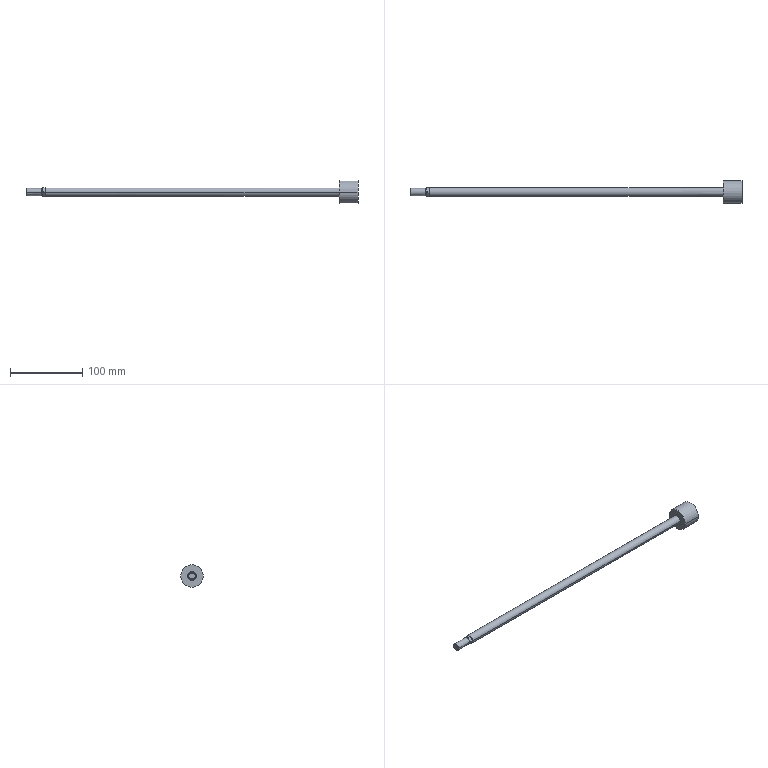Part | SolidWorks | features BaseBody 1 | 1 solid | 24 faces | box 458 x 31.1 x 31.1 mm | volume 67743 mm3 | plane 11 | cone 7 | cylinder 6 | commonest cylinder face diameters 10 x2 12 x2 31.1 x2
STEP:
#1=CARTESIAN_POINT('',(-48.,0.,-4.233));
#2=VERTEX_POINT('',#1);
#3=CARTESIAN_POINT('',(-48.,0.,4.233));
#4=VERTEX_POINT('',#3);
#5=CARTESIAN_POINT('',(-48.,0.,0.));
#6=DIRECTION('',(1.,0.,0.));
#7=DIRECTION('',(0.,0.,-1.));
#8=AXIS2_PLACEMENT_3D('',#5,#6,#7);
#9=CIRCLE('',#8,4.233);
#10=EDGE_CURVE('',#2,#4,#9,.T.);
#11=ORIENTED_EDGE('',*,*,#10,.F.);
#12=CARTESIAN_POINT('',(-48.,0.,0.));
#13=DIRECTION('',(1.,0.,0.));
#14=DIRECTION('',(0.,0.,-1.));
#15=AXIS2_PLACEMENT_3D('',#12,#13,#14);
#16=CIRCLE('',#15,4.233);
#17=EDGE_CURVE('',#4,#2,#16,.T.);
#18=ORIENTED_EDGE('',*,*,#17,.F.);
#19=EDGE_LOOP('',(#11,#18));
#20=FACE_OUTER_BOUND('',#19,.T.);
#21=CARTESIAN_POINT('',(-48.,0.,0.));
#22=DIRECTION('',(1.,0.,0.));
#23=DIRECTION('',(0.,-1.,0.));
#24=AXIS2_PLACEMENT_3D('',#21,#22,#23);
#25=PLANE('',#24);
#26=ADVANCED_FACE('',(#20),#25,.F.);
#27=CARTESIAN_POINT('',(410.,-15.55,0.));
#28=VERTEX_POINT('',#27);
#29=CARTESIAN_POINT('',(410.,15.55,0.));
#30=VERTEX_POINT('',#29);
#31=CARTESIAN_POINT('',(410.,0.,0.));
#32=DIRECTION('',(-1.,0.,0.));
#33=DIRECTION('',(0.,-1.,0.));
#34=AXIS2_PLACEMENT_3D('',#31,#32,#33);
#35=CIRCLE('',#34,15.55);
#36=EDGE_CURVE('',#28,#30,#35,.T.);
#37=ORIENTED_EDGE('',*,*,#36,.F.);
#38=CARTESIAN_POINT('',(410.,0.,0.));
#39=DIRECTION('',(-1.,0.,0.));
#40=DIRECTION('',(0.,-1.,0.));
#41=AXIS2_PLACEMENT_3D('',#38,#39,#40);
#42=CIRCLE('',#41,15.55);
#43=EDGE_CURVE('',#30,#28,#42,.T.);
#44=ORIENTED_EDGE('',*,*,#43,.F.);
#45=EDGE_LOOP('',(#37,#44));
#46=FACE_OUTER_BOUND('',#45,.T.);
#47=CARTESIAN_POINT('',(410.,15.55,0.));
#48=DIRECTION('',(-1.,0.,0.));
#49=DIRECTION('',(0.,0.,1.));
#50=AXIS2_PLACEMENT_3D('',#47,#48,#49);
#51=PLANE('',#50);
#52=ADVANCED_FACE('',(#46),#51,.F.);
#53=CARTESIAN_POINT('',(-47.233,0.,5.));
#54=VERTEX_POINT('',#53);
#55=CARTESIAN_POINT('',(-47.233,0.,5.));
#56=DIRECTION('',(0.7071,0.,0.7071));
#57=VECTOR('',#56,1000.);
#58=LINE('',#55,#57);
#59=EDGE_CURVE('',#4,#54,#58,.T.);
#60=ORIENTED_EDGE('',*,*,#59,.F.);
#61=ORIENTED_EDGE('',*,*,#17,.T.);
#62=CARTESIAN_POINT('',(-47.233,0.,-5.));
#63=VERTEX_POINT('',#62);
#64=CARTESIAN_POINT('',(-47.233,0.,-5.));
#65=DIRECTION('',(0.7071,0.,-0.7071));
#66=VECTOR('',#65,1000.);
#67=LINE('',#64,#66);
#68=EDGE_CURVE('',#2,#63,#67,.T.);
#69=ORIENTED_EDGE('',*,*,#68,.T.);
#70=CARTESIAN_POINT('',(-47.233,-5.,0.));
#71=VERTEX_POINT('',#70);
#72=CARTESIAN_POINT('',(-47.233,0.,0.));
#73=DIRECTION('',(1.,0.,0.));
#74=DIRECTION('',(0.,-1.,0.));
#75=AXIS2_PLACEMENT_3D('',#72,#73,#74);
#76=CIRCLE('',#75,5.);
#77=EDGE_CURVE('',#71,#63,#76,.T.);
#78=ORIENTED_EDGE('',*,*,#77,.F.);
#79=CARTESIAN_POINT('',(-47.233,0.,0.));
#80=DIRECTION('',(1.,0.,0.));
#81=DIRECTION('',(0.,-1.,0.));
#82=AXIS2_PLACEMENT_3D('',#79,#80,#81);
#83=CIRCLE('',#82,5.);
#84=EDGE_CURVE('',#54,#71,#83,.T.);
#85=ORIENTED_EDGE('',*,*,#84,.F.);
#86=EDGE_LOOP('',(#60,#61,#69,#78,#85));
#87=FACE_OUTER_BOUND('',#86,.T.);
#88=CARTESIAN_POINT('',(-47.233,0.,0.));
#89=DIRECTION('',(1.,0.,0.));
#90=DIRECTION('',(0.,0.,-1.));
#91=AXIS2_PLACEMENT_3D('',#88,#89,#90);
#92=CONICAL_SURFACE('',#91,5.,0.7854);
#93=ADVANCED_FACE('',(#87),#92,.T.);
#94=CARTESIAN_POINT('',(384.,15.55,0.));
#95=VERTEX_POINT('',#94);
#96=CARTESIAN_POINT('',(410.,15.55,0.));
#97=DIRECTION('',(-1.,0.,0.));
#98=VECTOR('',#97,1000.);
#99=LINE('',#96,#98);
#100=EDGE_CURVE('',#30,#95,#99,.T.);
#101=ORIENTED_EDGE('',*,*,#100,.F.);
#102=ORIENTED_EDGE('',*,*,#43,.T.);
#103=CARTESIAN_POINT('',(384.,-15.55,0.));
#104=VERTEX_POINT('',#103);
#105=CARTESIAN_POINT('',(410.,-15.55,0.));
#106=DIRECTION('',(-1.,0.,0.));
#107=VECTOR('',#106,1000.);
#108=LINE('',#105,#107);
#109=EDGE_CURVE('',#28,#104,#108,.T.);
#110=ORIENTED_EDGE('',*,*,#109,.T.);
#111=CARTESIAN_POINT('',(384.,0.,0.));
#112=DIRECTION('',(1.,0.,0.));
#113=DIRECTION('',(0.,-1.,0.));
#114=AXIS2_PLACEMENT_3D('',#111,#112,#113);
#115=CIRCLE('',#114,15.55);
#116=EDGE_CURVE('',#104,#95,#115,.T.);
#117=ORIENTED_EDGE('',*,*,#116,.T.);
#118=EDGE_LOOP('',(#101,#102,#110,#117));
#119=FACE_OUTER_BOUND('',#118,.T.);
#120=CARTESIAN_POINT('',(410.,0.,0.));
#121=DIRECTION('',(-1.,0.,0.));
#122=DIRECTION('',(0.,-1.,0.));
#123=AXIS2_PLACEMENT_3D('',#120,#121,#122);
#124=CYLINDRICAL_SURFACE('',#123,15.55);
#125=ADVANCED_FACE('',(#119),#124,.T.);
#126=CARTESIAN_POINT('',(-26.,5.,0.));
#127=VERTEX_POINT('',#126);
#128=CARTESIAN_POINT('',(-47.233,5.,0.));
#129=VERTEX_POINT('',#128);
#130=CARTESIAN_POINT('',(410.,5.,0.));
#131=DIRECTION('',(-1.,0.,0.));
#132=VECTOR('',#131,1000.);
#133=LINE('',#130,#132);
#134=EDGE_CURVE('',#127,#129,#133,.T.);
#135=ORIENTED_EDGE('',*,*,#134,.F.);
#136=CARTESIAN_POINT('',(-26.,3.536,-3.536));
#137=VERTEX_POINT('',#136);
#138=CARTESIAN_POINT('',(-26.,0.,0.));
#139=DIRECTION('',(1.,0.,0.));
#140=DIRECTION('',(0.,1.,0.));
#141=AXIS2_PLACEMENT_3D('',#138,#139,#140);
#142=CIRCLE('',#141,5.);
#143=EDGE_CURVE('',#137,#127,#142,.T.);
#144=ORIENTED_EDGE('',*,*,#143,.F.);
#145=CARTESIAN_POINT('',(-26.,0.,-5.));
#146=VERTEX_POINT('',#145);
#147=CARTESIAN_POINT('',(-26.,0.,0.));
#148=DIRECTION('',(1.,0.,0.));
#149=DIRECTION('',(0.,1.,0.));
#150=AXIS2_PLACEMENT_3D('',#147,#148,#149);
#151=CIRCLE('',#150,5.);
#152=EDGE_CURVE('',#146,#137,#151,.T.);
#153=ORIENTED_EDGE('',*,*,#152,.F.);
#154=CARTESIAN_POINT('',(-26.,-3.536,-3.536));
#155=VERTEX_POINT('',#154);
#156=CARTESIAN_POINT('',(-26.,0.,0.));
#157=DIRECTION('',(1.,0.,0.));
#158=DIRECTION('',(0.,1.,0.));
#159=AXIS2_PLACEMENT_3D('',#156,#157,#158);
#160=CIRCLE('',#159,5.);
#161=EDGE_CURVE('',#155,#146,#160,.T.);
#162=ORIENTED_EDGE('',*,*,#161,.F.);
#163=CARTESIAN_POINT('',(-26.,-5.,0.));
#164=VERTEX_POINT('',#163);
#165=CARTESIAN_POINT('',(-26.,0.,0.));
#166=DIRECTION('',(1.,0.,0.));
#167=DIRECTION('',(0.,1.,0.));
#168=AXIS2_PLACEMENT_3D('',#165,#166,#167);
#169=CIRCLE('',#168,5.);
#170=EDGE_CURVE('',#164,#155,#169,.T.);
#171=ORIENTED_EDGE('',*,*,#170,.F.);
#172=CARTESIAN_POINT('',(410.,-5.,0.));
#173=DIRECTION('',(-1.,0.,0.));
#174=VECTOR('',#173,1000.);
#175=LINE('',#172,#174);
#176=EDGE_CURVE('',#164,#71,#175,.T.);
#177=ORIENTED_EDGE('',*,*,#176,.T.);
#178=ORIENTED_EDGE('',*,*,#77,.T.);
#179=CARTESIAN_POINT('',(-47.233,0.,0.));
#180=DIRECTION('',(1.,0.,0.));
#181=DIRECTION('',(0.,-1.,0.));
#182=AXIS2_PLACEMENT_3D('',#179,#180,#181);
#183=CIRCLE('',#182,5.);
#184=EDGE_CURVE('',#63,#129,#183,.T.);
#185=ORIENTED_EDGE('',*,*,#184,.T.);
#186=EDGE_LOOP('',(#135,#144,#153,#162,#171,#177,#178,#185));
#187=FACE_OUTER_BOUND('',#186,.T.);
#188=CARTESIAN_POINT('',(410.,0.,0.));
#189=DIRECTION('',(-1.,0.,0.));
#190=DIRECTION('',(0.,-1.,0.));
#191=AXIS2_PLACEMENT_3D('',#188,#189,#190);
#192=CYLINDRICAL_SURFACE('',#191,5.);
#193=ADVANCED_FACE('',(#187),#192,.T.);
#194=CARTESIAN_POINT('',(384.,-6.,0.));
#195=VERTEX_POINT('',#194);
#196=CARTESIAN_POINT('',(384.,6.,0.));
#197=VERTEX_POINT('',#196);
#198=CARTESIAN_POINT('',(384.,0.,0.));
#199=DIRECTION('',(-1.,0.,0.));
#200=DIRECTION('',(0.,-1.,0.));
#201=AXIS2_PLACEMENT_3D('',#198,#199,#200);
#202=CIRCLE('',#201,6.);
#203=EDGE_CURVE('',#195,#197,#202,.T.);
#204=ORIENTED_EDGE('',*,*,#203,.F.);
#205=CARTESIAN_POINT('',(384.,0.,0.));
#206=DIRECTION('',(-1.,0.,0.));
#207=DIRECTION('',(0.,-1.,0.));
#208=AXIS2_PLACEMENT_3D('',#205,#206,#207);
#209=CIRCLE('',#208,6.);
#210=EDGE_CURVE('',#197,#195,#209,.T.);
#211=ORIENTED_EDGE('',*,*,#210,.F.);
#212=EDGE_LOOP('',(#204,#211));
#213=FACE_BOUND('',#212,.T.);
#214=ORIENTED_EDGE('',*,*,#116,.F.);
#215=CARTESIAN_POINT('',(384.,0.,0.));
#216=DIRECTION('',(1.,0.,0.));
#217=DIRECTION('',(0.,-1.,0.));
#218=AXIS2_PLACEMENT_3D('',#215,#216,#217);
#219=CIRCLE('',#218,15.55);
#220=EDGE_CURVE('',#95,#104,#219,.T.);
#221=ORIENTED_EDGE('',*,*,#220,.F.);
#222=EDGE_LOOP('',(#214,#221));
#223=FACE_OUTER_BOUND('',#222,.T.);
#224=CARTESIAN_POINT('',(384.,6.,0.));
#225=DIRECTION('',(1.,0.,0.));
#226=DIRECTION('',(0.,-1.,0.));
#227=AXIS2_PLACEMENT_3D('',#224,#225,#226);
#228=PLANE('',#227);
#229=ADVANCED_FACE('',(#213,#223),#228,.F.);
#230=CARTESIAN_POINT('',(-25.,0.,-6.));
#231=VERTEX_POINT('',#230);
#232=CARTESIAN_POINT('',(-25.,0.,-6.));
#233=DIRECTION('',(0.7071,0.,-0.7071));
#234=VECTOR('',#233,1000.);
#235=LINE('',#232,#234);
#236=EDGE_CURVE('',#146,#231,#235,.T.);
#237=ORIENTED_EDGE('',*,*,#236,.F.);
#238=ORIENTED_EDGE('',*,*,#152,.T.);
#239=CARTESIAN_POINT('',(-25.,1.19,-5.881));
#240=VERTEX_POINT('',#239);
#241=CARTESIAN_POINT('',(-25.,1.19,-5.881));
#242=CARTESIAN_POINT('',(-25.156,1.39,-5.682));
#243=CARTESIAN_POINT('',(-25.361,1.679,-5.392));
#244=CARTESIAN_POINT('',(-25.552,2.002,-5.069));
#245=CARTESIAN_POINT('',(-25.635,2.16,-4.911));
#246=CARTESIAN_POINT('',(-25.674,2.238,-4.833));
#247=CARTESIAN_POINT('',(-25.692,2.277,-4.795));
#248=CARTESIAN_POINT('',(-25.7,2.293,-4.778));
#249=CARTESIAN_POINT('',(-25.705,2.304,-4.767));
#250=CARTESIAN_POINT('',(-25.707,2.309,-4.763));
#251=CARTESIAN_POINT('',(-25.903,2.733,-4.338));
#252=CARTESIAN_POINT('',(-26.,3.14,-3.931));
#253=CARTESIAN_POINT('',(-26.,3.536,-3.536));
#254=B_SPLINE_CURVE_WITH_KNOTS('',3,(#241,#242,#243,#244,#245,#246,#247,#248,#249,#250,#251,#252,#253),.UNSPECIFIED.,.F.,.F.,(4,1,1,1,1,1,2,2,4),(0.,0.25,0.375,0.4375,0.4688,0.4844,0.4922,0.5,1.),.UNSPECIFIED.);
#255=EDGE_CURVE('',#240,#137,#254,.T.);
#256=ORIENTED_EDGE('',*,*,#255,.F.);
#257=CARTESIAN_POINT('',(-25.,0.,0.));
#258=DIRECTION('',(1.,0.,0.));
#259=DIRECTION('',(0.,-1.,0.));
#260=AXIS2_PLACEMENT_3D('',#257,#258,#259);
#261=CIRCLE('',#260,6.);
#262=EDGE_CURVE('',#231,#240,#261,.T.);
#263=ORIENTED_EDGE('',*,*,#262,.F.);
#264=EDGE_LOOP('',(#237,#238,#256,#263));
#265=FACE_OUTER_BOUND('',#264,.T.);
#266=CARTESIAN_POINT('',(-25.,0.,0.));
#267=DIRECTION('',(1.,0.,0.));
#268=DIRECTION('',(0.,0.,-1.));
#269=AXIS2_PLACEMENT_3D('',#266,#267,#268);
#270=CONICAL_SURFACE('',#269,6.,0.7854);
#271=ADVANCED_FACE('',(#265),#270,.T.);
#272=CARTESIAN_POINT('',(-21.4,1.19,-5.881));
#273=VERTEX_POINT('',#272);
#274=CARTESIAN_POINT('',(-21.4,5.881,-1.19));
#275=VERTEX_POINT('',#274);
#276=CARTESIAN_POINT('',(-21.4,1.19,-5.881));
#277=CARTESIAN_POINT('',(-20.025,3.628,-5.387));
#278=CARTESIAN_POINT('',(-20.025,5.387,-3.628));
#279=CARTESIAN_POINT('',(-21.4,5.881,-1.19));
#280=(BOUNDED_CURVE()B_SPLINE_CURVE(3,(#276,#277,#278,#279),.UNSPECIFIED.,.F.,.T.)B_SPLINE_CURVE_WITH_KNOTS((4,4),(2.556,3.727),.UNSPECIFIED.)CURVE()GEOMETRIC_REPRESENTATION_ITEM()RATIONAL_B_SPLINE_CURVE((1.,0.8889,0.8889,1.))REPRESENTATION_ITEM(''));
#281=EDGE_CURVE('',#273,#275,#280,.T.);
#282=ORIENTED_EDGE('',*,*,#281,.F.);
#283=CARTESIAN_POINT('',(-21.4,7.071,0.));
#284=DIRECTION('',(0.,-0.7071,-0.7071));
#285=VECTOR('',#284,1000.);
#286=LINE('',#283,#285);
#287=EDGE_CURVE('',#275,#273,#286,.T.);
#288=ORIENTED_EDGE('',*,*,#287,.F.);
#289=EDGE_LOOP('',(#282,#288));
#290=FACE_OUTER_BOUND('',#289,.T.);
#291=CARTESIAN_POINT('',(-21.4,7.071,0.));
#292=DIRECTION('',(-0.7071,0.5,-0.5));
#293=DIRECTION('',(-0.5774,0.,0.8165));
#294=AXIS2_PLACEMENT_3D('',#291,#292,#293);
#295=PLANE('',#294);
#296=ADVANCED_FACE('',(#290),#295,.T.);
#297=CARTESIAN_POINT('',(410.,1.19,-5.881));
#298=DIRECTION('',(1.,0.,0.));
#299=VECTOR('',#298,1000.);
#300=LINE('',#297,#299);
#301=EDGE_CURVE('',#240,#273,#300,.T.);
#302=ORIENTED_EDGE('',*,*,#301,.F.);
#303=ORIENTED_EDGE('',*,*,#255,.T.);
#304=CARTESIAN_POINT('',(-25.,5.881,-1.19));
#305=VERTEX_POINT('',#304);
#306=CARTESIAN_POINT('',(-25.,5.881,-1.19));
#307=CARTESIAN_POINT('',(-25.153,5.685,-1.386));
#308=CARTESIAN_POINT('',(-25.288,5.495,-1.576));
#309=CARTESIAN_POINT('',(-25.466,5.215,-1.856));
#310=CARTESIAN_POINT('',(-25.521,5.122,-1.949));
#311=CARTESIAN_POINT('',(-25.597,4.984,-2.087));
#312=CARTESIAN_POINT('',(-25.633,4.916,-2.155));
#313=CARTESIAN_POINT('',(-25.673,4.836,-2.235));
#314=CARTESIAN_POINT('',(-25.689,4.802,-2.269));
#315=CARTESIAN_POINT('',(-25.7,4.779,-2.292));
#316=CARTESIAN_POINT('',(-25.705,4.769,-2.302));
#317=CARTESIAN_POINT('',(-25.757,4.655,-2.416));
#318=CARTESIAN_POINT('',(-25.798,4.554,-2.517));
#319=CARTESIAN_POINT('',(-25.852,4.404,-2.667));
#320=CARTESIAN_POINT('',(-25.876,4.329,-2.742));
#321=CARTESIAN_POINT('',(-25.898,4.255,-2.817));
#322=CARTESIAN_POINT('',(-25.911,4.205,-2.866));
#323=CARTESIAN_POINT('',(-25.918,4.181,-2.89));
#324=CARTESIAN_POINT('',(-25.975,3.947,-3.124));
#325=CARTESIAN_POINT('',(-26.,3.742,-3.329));
#326=CARTESIAN_POINT('',(-26.,3.536,-3.536));
#327=B_SPLINE_CURVE_WITH_KNOTS('',3,(#306,#307,#308,#309,#310,#311,#312,#313,#314,#315,#316,#317,#318,#319,#320,#321,#322,#323,#324,#325,#326),.UNSPECIFIED.,.F.,.F.,(4,2,2,1,1,2,2,2,1,2,2,4),(0.,0.25,0.375,0.4375,0.4688,0.4844,0.5,0.625,0.6875,0.7188,0.75,1.),.UNSPECIFIED.);
#328=EDGE_CURVE('',#305,#137,#327,.T.);
#329=ORIENTED_EDGE('',*,*,#328,.F.);
#330=CARTESIAN_POINT('',(410.,5.881,-1.19));
#331=DIRECTION('',(-1.,0.,0.));
#332=VECTOR('',#331,1000.);
#333=LINE('',#330,#332);
#334=EDGE_CURVE('',#275,#305,#333,.T.);
#335=ORIENTED_EDGE('',*,*,#334,.F.);
#336=ORIENTED_EDGE('',*,*,#287,.T.);
#337=EDGE_LOOP('',(#302,#303,#329,#335,#336));
#338=FACE_OUTER_BOUND('',#337,.T.);
#339=CARTESIAN_POINT('',(-49.9,7.071,0.));
#340=DIRECTION('',(0.,0.7071,-0.7071));
#341=DIRECTION('',(-1.,0.,0.));
#342=AXIS2_PLACEMENT_3D('',#339,#340,#341);
#343=PLANE('',#342);
#344=ADVANCED_FACE('',(#338),#343,.T.);
#345=CARTESIAN_POINT('',(-25.,5.881,1.19));
#346=VERTEX_POINT('',#345);
#347=CARTESIAN_POINT('',(-26.,3.536,3.536));
#348=VERTEX_POINT('',#347);
#349=CARTESIAN_POINT('',(-25.,5.881,1.19));
#350=CARTESIAN_POINT('',(-25.156,5.682,1.39));
#351=CARTESIAN_POINT('',(-25.361,5.392,1.679));
#352=CARTESIAN_POINT('',(-25.552,5.069,2.002));
#353=CARTESIAN_POINT('',(-25.635,4.911,2.16));
#354=CARTESIAN_POINT('',(-25.674,4.833,2.238));
#355=CARTESIAN_POINT('',(-25.692,4.795,2.277));
#356=CARTESIAN_POINT('',(-25.7,4.778,2.293));
#357=CARTESIAN_POINT('',(-25.705,4.767,2.304));
#358=CARTESIAN_POINT('',(-25.707,4.763,2.309));
#359=CARTESIAN_POINT('',(-25.903,4.338,2.733));
#360=CARTESIAN_POINT('',(-26.,3.931,3.14));
#361=CARTESIAN_POINT('',(-26.,3.536,3.536));
#362=B_SPLINE_CURVE_WITH_KNOTS('',3,(#349,#350,#351,#352,#353,#354,#355,#356,#357,#358,#359,#360,#361),.UNSPECIFIED.,.F.,.F.,(4,1,1,1,1,1,2,2,4),(0.,0.25,0.375,0.4375,0.4688,0.4844,0.4922,0.5,1.),.UNSPECIFIED.);
#363=EDGE_CURVE('',#346,#348,#362,.T.);
#364=ORIENTED_EDGE('',*,*,#363,.F.);
#365=CARTESIAN_POINT('',(-25.,6.,0.));
#366=VERTEX_POINT('',#365);
#367=CARTESIAN_POINT('',(-25.,0.,0.));
#368=DIRECTION('',(1.,0.,0.));
#369=DIRECTION('',(0.,-1.,0.));
#370=AXIS2_PLACEMENT_3D('',#367,#368,#369);
#371=CIRCLE('',#370,6.);
#372=EDGE_CURVE('',#366,#346,#371,.T.);
#373=ORIENTED_EDGE('',*,*,#372,.F.);
#374=CARTESIAN_POINT('',(-25.,0.,0.));
#375=DIRECTION('',(1.,0.,0.));
#376=DIRECTION('',(0.,-1.,0.));
#377=AXIS2_PLACEMENT_3D('',#374,#375,#376);
#378=CIRCLE('',#377,6.);
#379=EDGE_CURVE('',#305,#366,#378,.T.);
#380=ORIENTED_EDGE('',*,*,#379,.F.);
#381=ORIENTED_EDGE('',*,*,#328,.T.);
#382=ORIENTED_EDGE('',*,*,#143,.T.);
#383=CARTESIAN_POINT('',(-26.,0.,0.));
#384=DIRECTION('',(1.,0.,0.));
#385=DIRECTION('',(0.,1.,0.));
#386=AXIS2_PLACEMENT_3D('',#383,#384,#385);
#387=CIRCLE('',#386,5.);
#388=EDGE_CURVE('',#127,#348,#387,.T.);
#389=ORIENTED_EDGE('',*,*,#388,.T.);
#390=EDGE_LOOP('',(#364,#373,#380,#381,#382,#389));
#391=FACE_OUTER_BOUND('',#390,.T.);
#392=CARTESIAN_POINT('',(-25.,0.,0.));
#393=DIRECTION('',(1.,0.,0.));
#394=DIRECTION('',(0.,0.,-1.));
#395=AXIS2_PLACEMENT_3D('',#392,#393,#394);
#396=CONICAL_SURFACE('',#395,6.,0.7854);
#397=ADVANCED_FACE('',(#391),#396,.T.);
#398=CARTESIAN_POINT('',(-21.4,5.881,1.19));
#399=VERTEX_POINT('',#398);
#400=CARTESIAN_POINT('',(-21.4,1.19,5.881));
#401=VERTEX_POINT('',#400);
#402=CARTESIAN_POINT('',(-21.4,5.881,1.19));
#403=CARTESIAN_POINT('',(-20.025,5.387,3.628));
#404=CARTESIAN_POINT('',(-20.025,3.628,5.387));
#405=CARTESIAN_POINT('',(-21.4,1.19,5.881));
#406=(BOUNDED_CURVE()B_SPLINE_CURVE(3,(#402,#403,#404,#405),.UNSPECIFIED.,.F.,.F.)B_SPLINE_CURVE_WITH_KNOTS((4,4),(2.556,3.727),.UNSPECIFIED.)CURVE()GEOMETRIC_REPRESENTATION_ITEM()RATIONAL_B_SPLINE_CURVE((1.,0.8889,0.8889,1.))REPRESENTATION_ITEM(''));
#407=EDGE_CURVE('',#399,#401,#406,.T.);
#408=ORIENTED_EDGE('',*,*,#407,.F.);
#409=CARTESIAN_POINT('',(-21.4,0.,7.071));
#410=DIRECTION('',(0.,0.7071,-0.7071));
#411=VECTOR('',#410,1000.);
#412=LINE('',#409,#411);
#413=EDGE_CURVE('',#401,#399,#412,.T.);
#414=ORIENTED_EDGE('',*,*,#413,.F.);
#415=EDGE_LOOP('',(#408,#414));
#416=FACE_OUTER_BOUND('',#415,.T.);
#417=CARTESIAN_POINT('',(-21.4,0.,7.071));
#418=DIRECTION('',(-0.7071,0.5,0.5));
#419=DIRECTION('',(0.5774,0.,0.8165));
#420=AXIS2_PLACEMENT_3D('',#417,#418,#419);
#421=PLANE('',#420);
#422=ADVANCED_FACE('',(#416),#421,.T.);
#423=ORIENTED_EDGE('',*,*,#413,.T.);
#424=CARTESIAN_POINT('',(410.,5.881,1.19));
#425=DIRECTION('',(1.,0.,0.));
#426=VECTOR('',#425,1000.);
#427=LINE('',#424,#426);
#428=EDGE_CURVE('',#346,#399,#427,.T.);
#429=ORIENTED_EDGE('',*,*,#428,.F.);
#430=ORIENTED_EDGE('',*,*,#363,.T.);
#431=CARTESIAN_POINT('',(-25.,1.19,5.881));
#432=VERTEX_POINT('',#431);
#433=CARTESIAN_POINT('',(-25.,1.19,5.881));
#434=CARTESIAN_POINT('',(-25.153,1.386,5.685));
#435=CARTESIAN_POINT('',(-25.288,1.576,5.495));
#436=CARTESIAN_POINT('',(-25.466,1.856,5.215));
#437=CARTESIAN_POINT('',(-25.521,1.949,5.122));
#438=CARTESIAN_POINT('',(-25.597,2.087,4.984));
#439=CARTESIAN_POINT('',(-25.633,2.155,4.916));
#440=CARTESIAN_POINT('',(-25.673,2.235,4.836));
#441=CARTESIAN_POINT('',(-25.689,2.269,4.802));
#442=CARTESIAN_POINT('',(-25.7,2.292,4.779));
#443=CARTESIAN_POINT('',(-25.705,2.302,4.769));
#444=CARTESIAN_POINT('',(-25.757,2.416,4.655));
#445=CARTESIAN_POINT('',(-25.798,2.517,4.554));
#446=CARTESIAN_POINT('',(-25.852,2.667,4.404));
#447=CARTESIAN_POINT('',(-25.876,2.742,4.329));
#448=CARTESIAN_POINT('',(-25.898,2.817,4.255));
#449=CARTESIAN_POINT('',(-25.911,2.866,4.205));
#450=CARTESIAN_POINT('',(-25.918,2.89,4.181));
#451=CARTESIAN_POINT('',(-25.975,3.124,3.947));
#452=CARTESIAN_POINT('',(-26.,3.329,3.742));
#453=CARTESIAN_POINT('',(-26.,3.536,3.536));
#454=B_SPLINE_CURVE_WITH_KNOTS('',3,(#433,#434,#435,#436,#437,#438,#439,#440,#441,#442,#443,#444,#445,#446,#447,#448,#449,#450,#451,#452,#453),.UNSPECIFIED.,.F.,.F.,(4,2,2,1,1,2,2,2,1,2,2,4),(0.,0.25,0.375,0.4375,0.4687,0.4844,0.5,0.625,0.6875,0.7187,0.75,1.),.UNSPECIFIED.);
#455=EDGE_CURVE('',#432,#348,#454,.T.);
#456=ORIENTED_EDGE('',*,*,#455,.F.);
#457=CARTESIAN_POINT('',(410.,1.19,5.881));
#458=DIRECTION('',(-1.,0.,0.));
#459=VECTOR('',#458,1000.);
#460=LINE('',#457,#459);
#461=EDGE_CURVE('',#401,#432,#460,.T.);
#462=ORIENTED_EDGE('',*,*,#461,.F.);
#463=EDGE_LOOP('',(#423,#429,#430,#456,#462));
#464=FACE_OUTER_BOUND('',#463,.T.);
#465=CARTESIAN_POINT('',(-49.9,0.,7.071));
#466=DIRECTION('',(0.,0.7071,0.7071));
#467=DIRECTION('',(1.,0.,0.));
#468=AXIS2_PLACEMENT_3D('',#465,#466,#467);
#469=PLANE('',#468);
#470=ADVANCED_FACE('',(#464),#469,.T.);
#471=CARTESIAN_POINT('',(-25.,-1.19,5.881));
#472=VERTEX_POINT('',#471);
#473=CARTESIAN_POINT('',(-26.,-3.536,3.536));
#474=VERTEX_POINT('',#473);
#475=CARTESIAN_POINT('',(-25.,-1.19,5.881));
#476=CARTESIAN_POINT('',(-25.156,-1.39,5.682));
#477=CARTESIAN_POINT('',(-25.361,-1.679,5.392));
#478=CARTESIAN_POINT('',(-25.552,-2.002,5.069));
#479=CARTESIAN_POINT('',(-25.635,-2.16,4.911));
#480=CARTESIAN_POINT('',(-25.674,-2.238,4.833));
#481=CARTESIAN_POINT('',(-25.692,-2.277,4.795));
#482=CARTESIAN_POINT('',(-25.7,-2.293,4.778));
#483=CARTESIAN_POINT('',(-25.705,-2.304,4.767));
#484=CARTESIAN_POINT('',(-25.707,-2.309,4.763));
#485=CARTESIAN_POINT('',(-25.903,-2.733,4.338));
#486=CARTESIAN_POINT('',(-26.,-3.14,3.931));
#487=CARTESIAN_POINT('',(-26.,-3.536,3.536));
#488=B_SPLINE_CURVE_WITH_KNOTS('',3,(#475,#476,#477,#478,#479,#480,#481,#482,#483,#484,#485,#486,#487),.UNSPECIFIED.,.F.,.F.,(4,1,1,1,1,1,2,2,4),(0.,0.25,0.375,0.4375,0.4688,0.4844,0.4922,0.5,1.),.UNSPECIFIED.);
#489=EDGE_CURVE('',#472,#474,#488,.T.);
#490=ORIENTED_EDGE('',*,*,#489,.F.);
#491=CARTESIAN_POINT('',(-25.,0.,0.));
#492=DIRECTION('',(1.,0.,0.));
#493=DIRECTION('',(0.,-1.,0.));
#494=AXIS2_PLACEMENT_3D('',#491,#492,#493);
#495=CIRCLE('',#494,6.);
#496=EDGE_CURVE('',#432,#472,#495,.T.);
#497=ORIENTED_EDGE('',*,*,#496,.F.);
#498=ORIENTED_EDGE('',*,*,#455,.T.);
#499=CARTESIAN_POINT('',(-26.,0.,0.));
#500=DIRECTION('',(1.,0.,0.));
#501=DIRECTION('',(0.,1.,0.));
#502=AXIS2_PLACEMENT_3D('',#499,#500,#501);
#503=CIRCLE('',#502,5.);
#504=EDGE_CURVE('',#348,#474,#503,.T.);
#505=ORIENTED_EDGE('',*,*,#504,.T.);
#506=EDGE_LOOP('',(#490,#497,#498,#505));
#507=FACE_OUTER_BOUND('',#506,.T.);
#508=CARTESIAN_POINT('',(-25.,0.,0.));
#509=DIRECTION('',(1.,0.,0.));
#510=DIRECTION('',(0.,0.,-1.));
#511=AXIS2_PLACEMENT_3D('',#508,#509,#510);
#512=CONICAL_SURFACE('',#511,6.,0.7854);
#513=ADVANCED_FACE('',(#507),#512,.T.);
#514=CARTESIAN_POINT('',(-21.4,-1.19,5.881));
#515=VERTEX_POINT('',#514);
#516=CARTESIAN_POINT('',(-21.4,-5.881,1.19));
#517=VERTEX_POINT('',#516);
#518=CARTESIAN_POINT('',(-21.4,-1.19,5.881));
#519=CARTESIAN_POINT('',(-20.025,-3.628,5.387));
#520=CARTESIAN_POINT('',(-20.025,-5.387,3.628));
#521=CARTESIAN_POINT('',(-21.4,-5.881,1.19));
#522=(BOUNDED_CURVE()B_SPLINE_CURVE(3,(#518,#519,#520,#521),.UNSPECIFIED.,.F.,.F.)B_SPLINE_CURVE_WITH_KNOTS((4,4),(2.556,3.727),.UNSPECIFIED.)CURVE()GEOMETRIC_REPRESENTATION_ITEM()RATIONAL_B_SPLINE_CURVE((1.,0.8889,0.8889,1.))REPRESENTATION_ITEM(''));
#523=EDGE_CURVE('',#515,#517,#522,.T.);
#524=ORIENTED_EDGE('',*,*,#523,.F.);
#525=CARTESIAN_POINT('',(-21.4,0.,7.071));
#526=DIRECTION('',(0.,0.7071,0.7071));
#527=VECTOR('',#526,1000.);
#528=LINE('',#525,#527);
#529=EDGE_CURVE('',#517,#515,#528,.T.);
#530=ORIENTED_EDGE('',*,*,#529,.F.);
#531=EDGE_LOOP('',(#524,#530));
#532=FACE_OUTER_BOUND('',#531,.T.);
#533=CARTESIAN_POINT('',(-20.4,-0.7071,7.778));
#534=DIRECTION('',(-0.7071,-0.5,0.5));
#535=DIRECTION('',(-0.5774,0.8165,0.));
#536=AXIS2_PLACEMENT_3D('',#533,#534,#535);
#537=PLANE('',#536);
#538=ADVANCED_FACE('',(#532),#537,.T.);
#539=CARTESIAN_POINT('',(410.,-1.19,5.881));
#540=DIRECTION('',(1.,0.,0.));
#541=VECTOR('',#540,1000.);
#542=LINE('',#539,#541);
#543=EDGE_CURVE('',#472,#515,#542,.T.);
#544=ORIENTED_EDGE('',*,*,#543,.F.);
#545=ORIENTED_EDGE('',*,*,#489,.T.);
#546=CARTESIAN_POINT('',(-25.,-5.881,1.19));
#547=VERTEX_POINT('',#546);
#548=CARTESIAN_POINT('',(-25.,-5.881,1.19));
#549=CARTESIAN_POINT('',(-25.153,-5.685,1.386));
#550=CARTESIAN_POINT('',(-25.288,-5.495,1.576));
#551=CARTESIAN_POINT('',(-25.466,-5.215,1.856));
#552=CARTESIAN_POINT('',(-25.521,-5.122,1.949));
#553=CARTESIAN_POINT('',(-25.597,-4.984,2.087));
#554=CARTESIAN_POINT('',(-25.633,-4.916,2.155));
#555=CARTESIAN_POINT('',(-25.673,-4.836,2.235));
#556=CARTESIAN_POINT('',(-25.689,-4.802,2.269));
#557=CARTESIAN_POINT('',(-25.7,-4.779,2.292));
#558=CARTESIAN_POINT('',(-25.705,-4.769,2.302));
#559=CARTESIAN_POINT('',(-25.757,-4.655,2.416));
#560=CARTESIAN_POINT('',(-25.798,-4.554,2.517));
#561=CARTESIAN_POINT('',(-25.852,-4.404,2.667));
#562=CARTESIAN_POINT('',(-25.876,-4.329,2.742));
#563=CARTESIAN_POINT('',(-25.898,-4.255,2.817));
#564=CARTESIAN_POINT('',(-25.911,-4.205,2.866));
#565=CARTESIAN_POINT('',(-25.918,-4.181,2.89));
#566=CARTESIAN_POINT('',(-25.975,-3.947,3.124));
#567=CARTESIAN_POINT('',(-26.,-3.742,3.329));
#568=CARTESIAN_POINT('',(-26.,-3.536,3.536));
#569=B_SPLINE_CURVE_WITH_KNOTS('',3,(#548,#549,#550,#551,#552,#553,#554,#555,#556,#557,#558,#559,#560,#561,#562,#563,#564,#565,#566,#567,#568),.UNSPECIFIED.,.F.,.F.,(4,2,2,1,1,2,2,2,1,2,2,4),(0.,0.25,0.375,0.4375,0.4687,0.4844,0.5,0.625,0.6875,0.7187,0.75,1.),.UNSPECIFIED.);
#570=EDGE_CURVE('',#547,#474,#569,.T.);
#571=ORIENTED_EDGE('',*,*,#570,.F.);
#572=CARTESIAN_POINT('',(410.,-5.881,1.19));
#573=DIRECTION('',(-1.,0.,0.));
#574=VECTOR('',#573,1000.);
#575=LINE('',#572,#574);
#576=EDGE_CURVE('',#517,#547,#575,.T.);
#577=ORIENTED_EDGE('',*,*,#576,.F.);
#578=ORIENTED_EDGE('',*,*,#529,.T.);
#579=EDGE_LOOP('',(#544,#545,#571,#577,#578));
#580=FACE_OUTER_BOUND('',#579,.T.);
#581=CARTESIAN_POINT('',(-21.4,0.,7.071));
#582=DIRECTION('',(0.,-0.7071,0.7071));
#583=DIRECTION('',(-1.,0.,0.));
#584=AXIS2_PLACEMENT_3D('',#581,#582,#583);
#585=PLANE('',#584);
#586=ADVANCED_FACE('',(#580),#585,.T.);
#587=ORIENTED_EDGE('',*,*,#570,.T.);
#588=CARTESIAN_POINT('',(-26.,0.,0.));
#589=DIRECTION('',(1.,0.,0.));
#590=DIRECTION('',(0.,1.,0.));
#591=AXIS2_PLACEMENT_3D('',#588,#589,#590);
#592=CIRCLE('',#591,5.);
#593=EDGE_CURVE('',#474,#164,#592,.T.);
#594=ORIENTED_EDGE('',*,*,#593,.T.);
#595=ORIENTED_EDGE('',*,*,#170,.T.);
#596=CARTESIAN_POINT('',(-25.,-5.881,-1.19));
#597=VERTEX_POINT('',#596);
#598=CARTESIAN_POINT('',(-25.,-5.881,-1.19));
#599=CARTESIAN_POINT('',(-25.156,-5.682,-1.39));
#600=CARTESIAN_POINT('',(-25.361,-5.392,-1.679));
#601=CARTESIAN_POINT('',(-25.552,-5.069,-2.002));
#602=CARTESIAN_POINT('',(-25.635,-4.911,-2.16));
#603=CARTESIAN_POINT('',(-25.674,-4.833,-2.238));
#604=CARTESIAN_POINT('',(-25.692,-4.795,-2.277));
#605=CARTESIAN_POINT('',(-25.7,-4.778,-2.293));
#606=CARTESIAN_POINT('',(-25.705,-4.767,-2.304));
#607=CARTESIAN_POINT('',(-25.707,-4.763,-2.309));
#608=CARTESIAN_POINT('',(-25.903,-4.338,-2.733));
#609=CARTESIAN_POINT('',(-26.,-3.931,-3.14));
#610=CARTESIAN_POINT('',(-26.,-3.536,-3.536));
#611=B_SPLINE_CURVE_WITH_KNOTS('',3,(#598,#599,#600,#601,#602,#603,#604,#605,#606,#607,#608,#609,#610),.UNSPECIFIED.,.F.,.F.,(4,1,1,1,1,1,2,2,4),(0.,0.25,0.375,0.4375,0.4688,0.4844,0.4922,0.5,1.),.UNSPECIFIED.);
#612=EDGE_CURVE('',#597,#155,#611,.T.);
#613=ORIENTED_EDGE('',*,*,#612,.F.);
#614=CARTESIAN_POINT('',(-25.,-6.,0.));
#615=VERTEX_POINT('',#614);
#616=CARTESIAN_POINT('',(-25.,0.,0.));
#617=DIRECTION('',(1.,0.,0.));
#618=DIRECTION('',(0.,-1.,0.));
#619=AXIS2_PLACEMENT_3D('',#616,#617,#618);
#620=CIRCLE('',#619,6.);
#621=EDGE_CURVE('',#615,#597,#620,.T.);
#622=ORIENTED_EDGE('',*,*,#621,.F.);
#623=CARTESIAN_POINT('',(-25.,0.,0.));
#624=DIRECTION('',(1.,0.,0.));
#625=DIRECTION('',(0.,-1.,0.));
#626=AXIS2_PLACEMENT_3D('',#623,#624,#625);
#627=CIRCLE('',#626,6.);
#628=EDGE_CURVE('',#547,#615,#627,.T.);
#629=ORIENTED_EDGE('',*,*,#628,.F.);
#630=EDGE_LOOP('',(#587,#594,#595,#613,#622,#629));
#631=FACE_OUTER_BOUND('',#630,.T.);
#632=CARTESIAN_POINT('',(-25.,0.,0.));
#633=DIRECTION('',(1.,0.,0.));
#634=DIRECTION('',(0.,0.,-1.));
#635=AXIS2_PLACEMENT_3D('',#632,#633,#634);
#636=CONICAL_SURFACE('',#635,6.,0.7854);
#637=ADVANCED_FACE('',(#631),#636,.T.);
#638=CARTESIAN_POINT('',(-21.4,-5.881,-1.19));
#639=VERTEX_POINT('',#638);
#640=CARTESIAN_POINT('',(-21.4,-1.19,-5.881));
#641=VERTEX_POINT('',#640);
#642=CARTESIAN_POINT('',(-21.4,-5.881,-1.19));
#643=DIRECTION('',(0.,0.7071,-0.7071));
#644=VECTOR('',#643,1000.);
#645=LINE('',#642,#644);
#646=EDGE_CURVE('',#639,#641,#645,.T.);
#647=ORIENTED_EDGE('',*,*,#646,.F.);
#648=CARTESIAN_POINT('',(410.,-5.881,-1.19));
#649=DIRECTION('',(1.,0.,0.));
#650=VECTOR('',#649,1000.);
#651=LINE('',#648,#650);
#652=EDGE_CURVE('',#597,#639,#651,.T.);
#653=ORIENTED_EDGE('',*,*,#652,.F.);
#654=ORIENTED_EDGE('',*,*,#612,.T.);
#655=CARTESIAN_POINT('',(-25.,-1.19,-5.881));
#656=VERTEX_POINT('',#655);
#657=CARTESIAN_POINT('',(-26.,-3.536,-3.536));
#658=CARTESIAN_POINT('',(-26.,-3.339,-3.732));
#659=CARTESIAN_POINT('',(-25.964,-3.04,-4.031));
#660=CARTESIAN_POINT('',(-25.86,-2.683,-4.388));
#661=CARTESIAN_POINT('',(-25.792,-2.503,-4.568));
#662=CARTESIAN_POINT('',(-25.754,-2.413,-4.658));
#663=CARTESIAN_POINT('',(-25.734,-2.367,-4.704));
#664=CARTESIAN_POINT('',(-25.725,-2.348,-4.723));
#665=CARTESIAN_POINT('',(-25.72,-2.335,-4.736));
#666=CARTESIAN_POINT('',(-25.716,-2.327,-4.744));
#667=CARTESIAN_POINT('',(-25.551,-1.969,-5.102));
#668=CARTESIAN_POINT('',(-25.314,-1.591,-5.48));
#669=CARTESIAN_POINT('',(-25.,-1.19,-5.881));
#670=B_SPLINE_CURVE_WITH_KNOTS('',3,(#657,#658,#659,#660,#661,#662,#663,#664,#665,#666,#667,#668,#669),.UNSPECIFIED.,.F.,.F.,(4,1,1,1,1,1,2,2,4),(0.,0.25,0.375,0.4375,0.4687,0.4844,0.4922,0.5,1.),.UNSPECIFIED.);
#671=EDGE_CURVE('',#155,#656,#670,.T.);
#672=ORIENTED_EDGE('',*,*,#671,.T.);
#673=CARTESIAN_POINT('',(410.,-1.19,-5.881));
#674=DIRECTION('',(-1.,0.,0.));
#675=VECTOR('',#674,1000.);
#676=LINE('',#673,#675);
#677=EDGE_CURVE('',#641,#656,#676,.T.);
#678=ORIENTED_EDGE('',*,*,#677,.F.);
#679=EDGE_LOOP('',(#647,#653,#654,#672,#678));
#680=FACE_OUTER_BOUND('',#679,.T.);
#681=CARTESIAN_POINT('',(-21.4,-7.071,0.));
#682=DIRECTION('',(0.,-0.7071,-0.7071));
#683=DIRECTION('',(0.,-0.7071,0.7071));
#684=AXIS2_PLACEMENT_3D('',#681,#682,#683);
#685=PLANE('',#684);
#686=ADVANCED_FACE('',(#680),#685,.T.);
#687=CARTESIAN_POINT('',(-21.4,-5.881,-1.19));
#688=CARTESIAN_POINT('',(-20.025,-5.387,-3.628));
#689=CARTESIAN_POINT('',(-20.025,-3.628,-5.387));
#690=CARTESIAN_POINT('',(-21.4,-1.19,-5.881));
#691=(BOUNDED_CURVE()B_SPLINE_CURVE(3,(#687,#688,#689,#690),.UNSPECIFIED.,.F.,.F.)B_SPLINE_CURVE_WITH_KNOTS((4,4),(2.556,3.727),.UNSPECIFIED.)CURVE()GEOMETRIC_REPRESENTATION_ITEM()RATIONAL_B_SPLINE_CURVE((1.,0.8889,0.8889,1.))REPRESENTATION_ITEM(''));
#692=EDGE_CURVE('',#639,#641,#691,.T.);
#693=ORIENTED_EDGE('',*,*,#692,.F.);
#694=ORIENTED_EDGE('',*,*,#646,.T.);
#695=EDGE_LOOP('',(#693,#694));
#696=FACE_OUTER_BOUND('',#695,.T.);
#697=CARTESIAN_POINT('',(-20.4,-7.778,-0.7071));
#698=DIRECTION('',(-0.7071,-0.5,-0.5));
#699=DIRECTION('',(-0.5774,0.8165,0.));
#700=AXIS2_PLACEMENT_3D('',#697,#698,#699);
#701=PLANE('',#700);
#702=ADVANCED_FACE('',(#696),#701,.T.);
#703=CARTESIAN_POINT('',(410.,6.,0.));
#704=DIRECTION('',(-1.,0.,0.));
#705=VECTOR('',#704,1000.);
#706=LINE('',#703,#705);
#707=EDGE_CURVE('',#197,#366,#706,.T.);
#708=ORIENTED_EDGE('',*,*,#707,.F.);
#709=ORIENTED_EDGE('',*,*,#210,.T.);
#710=CARTESIAN_POINT('',(410.,-6.,0.));
#711=DIRECTION('',(-1.,0.,0.));
#712=VECTOR('',#711,1000.);
#713=LINE('',#710,#712);
#714=EDGE_CURVE('',#195,#615,#713,.T.);
#715=ORIENTED_EDGE('',*,*,#714,.T.);
#716=ORIENTED_EDGE('',*,*,#621,.T.);
#717=ORIENTED_EDGE('',*,*,#652,.T.);
#718=ORIENTED_EDGE('',*,*,#692,.T.);
#719=ORIENTED_EDGE('',*,*,#677,.T.);
#720=CARTESIAN_POINT('',(-25.,0.,0.));
#721=DIRECTION('',(1.,0.,0.));
#722=DIRECTION('',(0.,-1.,0.));
#723=AXIS2_PLACEMENT_3D('',#720,#721,#722);
#724=CIRCLE('',#723,6.);
#725=EDGE_CURVE('',#656,#231,#724,.T.);
#726=ORIENTED_EDGE('',*,*,#725,.T.);
#727=ORIENTED_EDGE('',*,*,#262,.T.);
#728=ORIENTED_EDGE('',*,*,#301,.T.);
#729=ORIENTED_EDGE('',*,*,#281,.T.);
#730=ORIENTED_EDGE('',*,*,#334,.T.);
#731=ORIENTED_EDGE('',*,*,#379,.T.);
#732=EDGE_LOOP('',(#708,#709,#715,#716,#717,#718,#719,#726,#727,#728,#729,#730,#731));
#733=FACE_OUTER_BOUND('',#732,.T.);
#734=CARTESIAN_POINT('',(410.,0.,0.));
#735=DIRECTION('',(-1.,0.,0.));
#736=DIRECTION('',(0.,-1.,0.));
#737=AXIS2_PLACEMENT_3D('',#734,#735,#736);
#738=CYLINDRICAL_SURFACE('',#737,6.);
#739=ADVANCED_FACE('',(#733),#738,.T.);
#740=ORIENTED_EDGE('',*,*,#10,.T.);
#741=ORIENTED_EDGE('',*,*,#59,.T.);
#742=CARTESIAN_POINT('',(-47.233,0.,0.));
#743=DIRECTION('',(1.,0.,0.));
#744=DIRECTION('',(0.,-1.,0.));
#745=AXIS2_PLACEMENT_3D('',#742,#743,#744);
#746=CIRCLE('',#745,5.);
#747=EDGE_CURVE('',#129,#54,#746,.T.);
#748=ORIENTED_EDGE('',*,*,#747,.F.);
#749=ORIENTED_EDGE('',*,*,#184,.F.);
#750=ORIENTED_EDGE('',*,*,#68,.F.);
#751=EDGE_LOOP('',(#740,#741,#748,#749,#750));
#752=FACE_OUTER_BOUND('',#751,.T.);
#753=CARTESIAN_POINT('',(-47.233,0.,0.));
#754=DIRECTION('',(1.,0.,0.));
#755=DIRECTION('',(0.,0.,-1.));
#756=AXIS2_PLACEMENT_3D('',#753,#754,#755);
#757=CONICAL_SURFACE('',#756,5.,0.7854);
#758=ADVANCED_FACE('',(#752),#757,.T.);
#759=ORIENTED_EDGE('',*,*,#36,.T.);
#760=ORIENTED_EDGE('',*,*,#100,.T.);
#761=ORIENTED_EDGE('',*,*,#220,.T.);
#762=ORIENTED_EDGE('',*,*,#109,.F.);
#763=EDGE_LOOP('',(#759,#760,#761,#762));
#764=FACE_OUTER_BOUND('',#763,.T.);
#765=CARTESIAN_POINT('',(410.,0.,0.));
#766=DIRECTION('',(-1.,0.,0.));
#767=DIRECTION('',(0.,-1.,0.));
#768=AXIS2_PLACEMENT_3D('',#765,#766,#767);
#769=CYLINDRICAL_SURFACE('',#768,15.55);
#770=ADVANCED_FACE('',(#764),#769,.T.);
#771=ORIENTED_EDGE('',*,*,#388,.F.);
#772=ORIENTED_EDGE('',*,*,#134,.T.);
#773=ORIENTED_EDGE('',*,*,#747,.T.);
#774=ORIENTED_EDGE('',*,*,#84,.T.);
#775=ORIENTED_EDGE('',*,*,#176,.F.);
#776=ORIENTED_EDGE('',*,*,#593,.F.);
#777=ORIENTED_EDGE('',*,*,#504,.F.);
#778=EDGE_LOOP('',(#771,#772,#773,#774,#775,#776,#777));
#779=FACE_OUTER_BOUND('',#778,.T.);
#780=CARTESIAN_POINT('',(410.,0.,0.));
#781=DIRECTION('',(-1.,0.,0.));
#782=DIRECTION('',(0.,-1.,0.));
#783=AXIS2_PLACEMENT_3D('',#780,#781,#782);
#784=CYLINDRICAL_SURFACE('',#783,5.);
#785=ADVANCED_FACE('',(#779),#784,.T.);
#786=ORIENTED_EDGE('',*,*,#161,.T.);
#787=ORIENTED_EDGE('',*,*,#236,.T.);
#788=ORIENTED_EDGE('',*,*,#725,.F.);
#789=ORIENTED_EDGE('',*,*,#671,.F.);
#790=EDGE_LOOP('',(#786,#787,#788,#789));
#791=FACE_OUTER_BOUND('',#790,.T.);
#792=CARTESIAN_POINT('',(-25.,0.,0.));
#793=DIRECTION('',(1.,0.,0.));
#794=DIRECTION('',(0.,0.,-1.));
#795=AXIS2_PLACEMENT_3D('',#792,#793,#794);
#796=CONICAL_SURFACE('',#795,6.,0.7854);
#797=ADVANCED_FACE('',(#791),#796,.T.);
#798=ORIENTED_EDGE('',*,*,#203,.T.);
#799=ORIENTED_EDGE('',*,*,#707,.T.);
#800=ORIENTED_EDGE('',*,*,#372,.T.);
#801=ORIENTED_EDGE('',*,*,#428,.T.);
#802=ORIENTED_EDGE('',*,*,#407,.T.);
#803=ORIENTED_EDGE('',*,*,#461,.T.);
#804=ORIENTED_EDGE('',*,*,#496,.T.);
#805=ORIENTED_EDGE('',*,*,#543,.T.);
#806=ORIENTED_EDGE('',*,*,#523,.T.);
#807=ORIENTED_EDGE('',*,*,#576,.T.);
#808=ORIENTED_EDGE('',*,*,#628,.T.);
#809=ORIENTED_EDGE('',*,*,#714,.F.);
#810=EDGE_LOOP('',(#798,#799,#800,#801,#802,#803,#804,#805,#806,#807,#808,#809));
#811=FACE_OUTER_BOUND('',#810,.T.);
#812=CARTESIAN_POINT('',(410.,0.,0.));
#813=DIRECTION('',(-1.,0.,0.));
#814=DIRECTION('',(0.,-1.,0.));
#815=AXIS2_PLACEMENT_3D('',#812,#813,#814);
#816=CYLINDRICAL_SURFACE('',#815,6.);
#817=ADVANCED_FACE('',(#811),#816,.T.);
#818=CLOSED_SHELL('',(#26,#52,#93,#125,#193,#229,#271,#296,#344,#397,#422,#470,#513,#538,#586,#637,#686,#702,#739,#758,#770,#785,#797,#817));
#819=MANIFOLD_SOLID_BREP('',#818);
#820=CARTESIAN_POINT('',(0.,0.,0.));
#821=DIRECTION('',(0.,0.,1.));
#822=DIRECTION('',(1.,0.,0.));
#823=AXIS2_PLACEMENT_3D('',#820,#821,#822);
#824=(LENGTH_UNIT()NAMED_UNIT(*)SI_UNIT(.MILLI.,.METRE.));
#825=UNCERTAINTY_MEASURE_WITH_UNIT(LENGTH_MEASURE(0.00001),#824,'','');
#826=(NAMED_UNIT(*)PLANE_ANGLE_UNIT()SI_UNIT($,.RADIAN.));
#827=(NAMED_UNIT(*)SI_UNIT($,.STERADIAN.)SOLID_ANGLE_UNIT());
#828=(GEOMETRIC_REPRESENTATION_CONTEXT(3)GLOBAL_UNCERTAINTY_ASSIGNED_CONTEXT((#825))GLOBAL_UNIT_ASSIGNED_CONTEXT((#824,#826,#827))REPRESENTATION_CONTEXT('',''));
#829=ADVANCED_BREP_SHAPE_REPRESENTATION('',(#819,#823),#828);